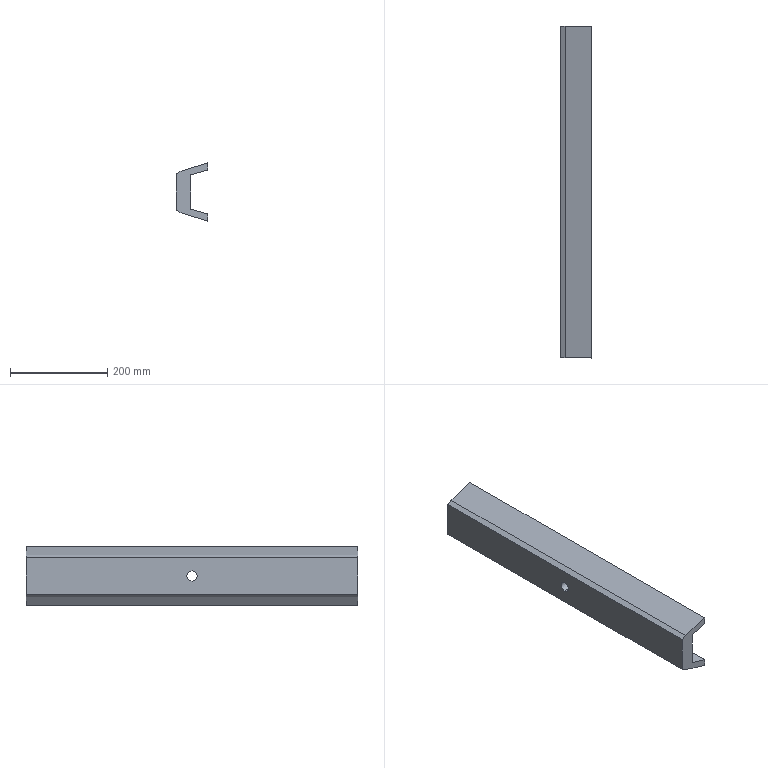Part | SolidWorks | features Extrusion 1, ICE 1 | 1 solid | 14 faces | box 65 x 682 x 120 mm | volume 2487309 mm3 | plane 12 | cylinder 2 | commonest cylinder face diameters 21 x2
STEP:
#1=CARTESIAN_POINT('',(30.,0.,-10.5));
#2=VERTEX_POINT('',#1);
#3=CARTESIAN_POINT('',(30.,0.,10.5));
#4=VERTEX_POINT('',#3);
#5=CARTESIAN_POINT('',(30.,0.,0.));
#6=DIRECTION('',(-1.,0.,0.));
#7=DIRECTION('',(0.,0.,1.));
#8=AXIS2_PLACEMENT_3D('',#5,#6,#7);
#9=CIRCLE('',#8,10.5);
#10=EDGE_CURVE('',#2,#4,#9,.T.);
#11=ORIENTED_EDGE('',*,*,#10,.F.);
#12=CARTESIAN_POINT('',(0.,0.,-10.5));
#13=VERTEX_POINT('',#12);
#14=CARTESIAN_POINT('',(95.,0.,-10.5));
#15=DIRECTION('',(-1.,0.,0.));
#16=VECTOR('',#15,1000.);
#17=LINE('',#14,#16);
#18=EDGE_CURVE('',#2,#13,#17,.T.);
#19=ORIENTED_EDGE('',*,*,#18,.T.);
#20=CARTESIAN_POINT('',(0.,0.,10.5));
#21=VERTEX_POINT('',#20);
#22=CARTESIAN_POINT('',(0.,0.,0.));
#23=DIRECTION('',(-1.,0.,0.));
#24=DIRECTION('',(0.,0.,1.));
#25=AXIS2_PLACEMENT_3D('',#22,#23,#24);
#26=CIRCLE('',#25,10.5);
#27=EDGE_CURVE('',#13,#21,#26,.T.);
#28=ORIENTED_EDGE('',*,*,#27,.T.);
#29=CARTESIAN_POINT('',(95.,0.,10.5));
#30=DIRECTION('',(-1.,0.,0.));
#31=VECTOR('',#30,1000.);
#32=LINE('',#29,#31);
#33=EDGE_CURVE('',#4,#21,#32,.T.);
#34=ORIENTED_EDGE('',*,*,#33,.F.);
#35=EDGE_LOOP('',(#11,#19,#28,#34));
#36=FACE_OUTER_BOUND('',#35,.T.);
#37=CARTESIAN_POINT('',(95.,0.,0.));
#38=DIRECTION('',(-1.,0.,0.));
#39=DIRECTION('',(0.,0.,1.));
#40=AXIS2_PLACEMENT_3D('',#37,#38,#39);
#41=CYLINDRICAL_SURFACE('',#40,10.5);
#42=ADVANCED_FACE('',(#36),#41,.F.);
#43=CARTESIAN_POINT('',(65.,-341.,45.));
#44=VERTEX_POINT('',#43);
#45=CARTESIAN_POINT('',(30.,-341.,35.));
#46=VERTEX_POINT('',#45);
#47=CARTESIAN_POINT('',(65.,-341.,45.));
#48=DIRECTION('',(-0.9615,0.,-0.2747));
#49=VECTOR('',#48,1000.);
#50=LINE('',#47,#49);
#51=EDGE_CURVE('',#44,#46,#50,.T.);
#52=ORIENTED_EDGE('',*,*,#51,.T.);
#53=CARTESIAN_POINT('',(30.,341.,35.));
#54=VERTEX_POINT('',#53);
#55=CARTESIAN_POINT('',(30.,341.,35.));
#56=DIRECTION('',(0.,-1.,0.));
#57=VECTOR('',#56,1000.);
#58=LINE('',#55,#57);
#59=EDGE_CURVE('',#54,#46,#58,.T.);
#60=ORIENTED_EDGE('',*,*,#59,.F.);
#61=CARTESIAN_POINT('',(65.,341.,45.));
#62=VERTEX_POINT('',#61);
#63=CARTESIAN_POINT('',(65.,341.,45.));
#64=DIRECTION('',(-0.9615,0.,-0.2747));
#65=VECTOR('',#64,1000.);
#66=LINE('',#63,#65);
#67=EDGE_CURVE('',#62,#54,#66,.T.);
#68=ORIENTED_EDGE('',*,*,#67,.F.);
#69=CARTESIAN_POINT('',(65.,341.,45.));
#70=DIRECTION('',(0.,-1.,0.));
#71=VECTOR('',#70,1000.);
#72=LINE('',#69,#71);
#73=EDGE_CURVE('',#62,#44,#72,.T.);
#74=ORIENTED_EDGE('',*,*,#73,.T.);
#75=EDGE_LOOP('',(#52,#60,#68,#74));
#76=FACE_OUTER_BOUND('',#75,.T.);
#77=CARTESIAN_POINT('',(65.,341.,45.));
#78=DIRECTION('',(-0.2747,0.,0.9615));
#79=DIRECTION('',(0.9615,0.,0.2747));
#80=AXIS2_PLACEMENT_3D('',#77,#78,#79);
#81=PLANE('',#80);
#82=ADVANCED_FACE('',(#76),#81,.F.);
#83=CARTESIAN_POINT('',(30.,0.,0.));
#84=DIRECTION('',(-1.,0.,0.));
#85=DIRECTION('',(0.,0.,1.));
#86=AXIS2_PLACEMENT_3D('',#83,#84,#85);
#87=CIRCLE('',#86,10.5);
#88=EDGE_CURVE('',#4,#2,#87,.T.);
#89=ORIENTED_EDGE('',*,*,#88,.T.);
#90=ORIENTED_EDGE('',*,*,#10,.T.);
#91=EDGE_LOOP('',(#89,#90));
#92=FACE_BOUND('',#91,.T.);
#93=CARTESIAN_POINT('',(30.,-341.,-35.));
#94=VERTEX_POINT('',#93);
#95=CARTESIAN_POINT('',(30.,-341.,-35.));
#96=DIRECTION('',(0.,0.,-1.));
#97=VECTOR('',#96,1000.);
#98=LINE('',#95,#97);
#99=EDGE_CURVE('',#46,#94,#98,.T.);
#100=ORIENTED_EDGE('',*,*,#99,.T.);
#101=CARTESIAN_POINT('',(30.,341.,-35.));
#102=VERTEX_POINT('',#101);
#103=CARTESIAN_POINT('',(30.,341.,-35.));
#104=DIRECTION('',(0.,-1.,0.));
#105=VECTOR('',#104,1000.);
#106=LINE('',#103,#105);
#107=EDGE_CURVE('',#102,#94,#106,.T.);
#108=ORIENTED_EDGE('',*,*,#107,.F.);
#109=CARTESIAN_POINT('',(30.,341.,-35.));
#110=DIRECTION('',(0.,0.,-1.));
#111=VECTOR('',#110,1000.);
#112=LINE('',#109,#111);
#113=EDGE_CURVE('',#54,#102,#112,.T.);
#114=ORIENTED_EDGE('',*,*,#113,.F.);
#115=ORIENTED_EDGE('',*,*,#59,.T.);
#116=EDGE_LOOP('',(#100,#108,#114,#115));
#117=FACE_OUTER_BOUND('',#116,.T.);
#118=CARTESIAN_POINT('',(30.,341.,-35.));
#119=DIRECTION('',(-1.,0.,0.));
#120=DIRECTION('',(0.,0.,1.));
#121=AXIS2_PLACEMENT_3D('',#118,#119,#120);
#122=PLANE('',#121);
#123=ADVANCED_FACE('',(#92,#117),#122,.F.);
#124=CARTESIAN_POINT('',(65.,-341.,-45.));
#125=VERTEX_POINT('',#124);
#126=CARTESIAN_POINT('',(65.,-341.,-45.));
#127=DIRECTION('',(0.9615,0.,-0.2747));
#128=VECTOR('',#127,1000.);
#129=LINE('',#126,#128);
#130=EDGE_CURVE('',#94,#125,#129,.T.);
#131=ORIENTED_EDGE('',*,*,#130,.T.);
#132=CARTESIAN_POINT('',(65.,341.,-45.));
#133=VERTEX_POINT('',#132);
#134=CARTESIAN_POINT('',(65.,341.,-45.));
#135=DIRECTION('',(0.,-1.,0.));
#136=VECTOR('',#135,1000.);
#137=LINE('',#134,#136);
#138=EDGE_CURVE('',#133,#125,#137,.T.);
#139=ORIENTED_EDGE('',*,*,#138,.F.);
#140=CARTESIAN_POINT('',(65.,341.,-45.));
#141=DIRECTION('',(0.9615,0.,-0.2747));
#142=VECTOR('',#141,1000.);
#143=LINE('',#140,#142);
#144=EDGE_CURVE('',#102,#133,#143,.T.);
#145=ORIENTED_EDGE('',*,*,#144,.F.);
#146=ORIENTED_EDGE('',*,*,#107,.T.);
#147=EDGE_LOOP('',(#131,#139,#145,#146));
#148=FACE_OUTER_BOUND('',#147,.T.);
#149=CARTESIAN_POINT('',(65.,341.,-45.));
#150=DIRECTION('',(-0.2747,0.,-0.9615));
#151=DIRECTION('',(-0.9615,0.,0.2747));
#152=AXIS2_PLACEMENT_3D('',#149,#150,#151);
#153=PLANE('',#152);
#154=ADVANCED_FACE('',(#148),#153,.F.);
#155=CARTESIAN_POINT('',(65.,-341.,-60.));
#156=VERTEX_POINT('',#155);
#157=CARTESIAN_POINT('',(65.,-341.,-60.));
#158=DIRECTION('',(0.,0.,-1.));
#159=VECTOR('',#158,1000.);
#160=LINE('',#157,#159);
#161=EDGE_CURVE('',#125,#156,#160,.T.);
#162=ORIENTED_EDGE('',*,*,#161,.T.);
#163=CARTESIAN_POINT('',(65.,341.,-60.));
#164=VERTEX_POINT('',#163);
#165=CARTESIAN_POINT('',(65.,341.,-60.));
#166=DIRECTION('',(0.,-1.,0.));
#167=VECTOR('',#166,1000.);
#168=LINE('',#165,#167);
#169=EDGE_CURVE('',#164,#156,#168,.T.);
#170=ORIENTED_EDGE('',*,*,#169,.F.);
#171=CARTESIAN_POINT('',(65.,341.,-60.));
#172=DIRECTION('',(0.,0.,-1.));
#173=VECTOR('',#172,1000.);
#174=LINE('',#171,#173);
#175=EDGE_CURVE('',#133,#164,#174,.T.);
#176=ORIENTED_EDGE('',*,*,#175,.F.);
#177=ORIENTED_EDGE('',*,*,#138,.T.);
#178=EDGE_LOOP('',(#162,#170,#176,#177));
#179=FACE_OUTER_BOUND('',#178,.T.);
#180=CARTESIAN_POINT('',(65.,341.,-60.));
#181=DIRECTION('',(-1.,0.,0.));
#182=DIRECTION('',(0.,0.,1.));
#183=AXIS2_PLACEMENT_3D('',#180,#181,#182);
#184=PLANE('',#183);
#185=ADVANCED_FACE('',(#179),#184,.F.);
#186=CARTESIAN_POINT('',(10.,-341.,-42.882));
#187=VERTEX_POINT('',#186);
#188=CARTESIAN_POINT('',(10.,-341.,-42.882));
#189=DIRECTION('',(-0.9548,0.,0.2972));
#190=VECTOR('',#189,1000.);
#191=LINE('',#188,#190);
#192=EDGE_CURVE('',#156,#187,#191,.T.);
#193=ORIENTED_EDGE('',*,*,#192,.T.);
#194=CARTESIAN_POINT('',(10.,341.,-42.882));
#195=VERTEX_POINT('',#194);
#196=CARTESIAN_POINT('',(10.,341.,-42.882));
#197=DIRECTION('',(0.,-1.,0.));
#198=VECTOR('',#197,1000.);
#199=LINE('',#196,#198);
#200=EDGE_CURVE('',#195,#187,#199,.T.);
#201=ORIENTED_EDGE('',*,*,#200,.F.);
#202=CARTESIAN_POINT('',(10.,341.,-42.882));
#203=DIRECTION('',(-0.9548,0.,0.2972));
#204=VECTOR('',#203,1000.);
#205=LINE('',#202,#204);
#206=EDGE_CURVE('',#164,#195,#205,.T.);
#207=ORIENTED_EDGE('',*,*,#206,.F.);
#208=ORIENTED_EDGE('',*,*,#169,.T.);
#209=EDGE_LOOP('',(#193,#201,#207,#208));
#210=FACE_OUTER_BOUND('',#209,.T.);
#211=CARTESIAN_POINT('',(10.,341.,-42.882));
#212=DIRECTION('',(0.2972,0.,0.9548));
#213=DIRECTION('',(0.9548,0.,-0.2972));
#214=AXIS2_PLACEMENT_3D('',#211,#212,#213);
#215=PLANE('',#214);
#216=ADVANCED_FACE('',(#210),#215,.F.);
#217=CARTESIAN_POINT('',(0.,-341.,-37.5));
#218=VERTEX_POINT('',#217);
#219=CARTESIAN_POINT('',(0.,-341.,-37.5));
#220=DIRECTION('',(-0.8806,0.,0.4739));
#221=VECTOR('',#220,1000.);
#222=LINE('',#219,#221);
#223=EDGE_CURVE('',#187,#218,#222,.T.);
#224=ORIENTED_EDGE('',*,*,#223,.T.);
#225=CARTESIAN_POINT('',(0.,341.,-37.5));
#226=VERTEX_POINT('',#225);
#227=CARTESIAN_POINT('',(0.,341.,-37.5));
#228=DIRECTION('',(0.,-1.,0.));
#229=VECTOR('',#228,1000.);
#230=LINE('',#227,#229);
#231=EDGE_CURVE('',#226,#218,#230,.T.);
#232=ORIENTED_EDGE('',*,*,#231,.F.);
#233=CARTESIAN_POINT('',(0.,341.,-37.5));
#234=DIRECTION('',(-0.8806,0.,0.4739));
#235=VECTOR('',#234,1000.);
#236=LINE('',#233,#235);
#237=EDGE_CURVE('',#195,#226,#236,.T.);
#238=ORIENTED_EDGE('',*,*,#237,.F.);
#239=ORIENTED_EDGE('',*,*,#200,.T.);
#240=EDGE_LOOP('',(#224,#232,#238,#239));
#241=FACE_OUTER_BOUND('',#240,.T.);
#242=CARTESIAN_POINT('',(0.,341.,-37.5));
#243=DIRECTION('',(0.4739,0.,0.8806));
#244=DIRECTION('',(0.8806,0.,-0.4739));
#245=AXIS2_PLACEMENT_3D('',#242,#243,#244);
#246=PLANE('',#245);
#247=ADVANCED_FACE('',(#241),#246,.F.);
#248=CARTESIAN_POINT('',(0.,0.,0.));
#249=DIRECTION('',(-1.,0.,0.));
#250=DIRECTION('',(0.,0.,1.));
#251=AXIS2_PLACEMENT_3D('',#248,#249,#250);
#252=CIRCLE('',#251,10.5);
#253=EDGE_CURVE('',#21,#13,#252,.T.);
#254=ORIENTED_EDGE('',*,*,#253,.F.);
#255=ORIENTED_EDGE('',*,*,#27,.F.);
#256=EDGE_LOOP('',(#254,#255));
#257=FACE_BOUND('',#256,.T.);
#258=CARTESIAN_POINT('',(0.,-341.,37.5));
#259=VERTEX_POINT('',#258);
#260=CARTESIAN_POINT('',(0.,-341.,37.5));
#261=DIRECTION('',(0.,0.,1.));
#262=VECTOR('',#261,1000.);
#263=LINE('',#260,#262);
#264=EDGE_CURVE('',#218,#259,#263,.T.);
#265=ORIENTED_EDGE('',*,*,#264,.T.);
#266=CARTESIAN_POINT('',(0.,341.,37.5));
#267=VERTEX_POINT('',#266);
#268=CARTESIAN_POINT('',(0.,341.,37.5));
#269=DIRECTION('',(0.,-1.,0.));
#270=VECTOR('',#269,1000.);
#271=LINE('',#268,#270);
#272=EDGE_CURVE('',#267,#259,#271,.T.);
#273=ORIENTED_EDGE('',*,*,#272,.F.);
#274=CARTESIAN_POINT('',(0.,341.,37.5));
#275=DIRECTION('',(0.,0.,1.));
#276=VECTOR('',#275,1000.);
#277=LINE('',#274,#276);
#278=EDGE_CURVE('',#226,#267,#277,.T.);
#279=ORIENTED_EDGE('',*,*,#278,.F.);
#280=ORIENTED_EDGE('',*,*,#231,.T.);
#281=EDGE_LOOP('',(#265,#273,#279,#280));
#282=FACE_OUTER_BOUND('',#281,.T.);
#283=CARTESIAN_POINT('',(0.,341.,37.5));
#284=DIRECTION('',(1.,0.,0.));
#285=DIRECTION('',(0.,0.,-1.));
#286=AXIS2_PLACEMENT_3D('',#283,#284,#285);
#287=PLANE('',#286);
#288=ADVANCED_FACE('',(#257,#282),#287,.F.);
#289=CARTESIAN_POINT('',(10.,-341.,42.882));
#290=VERTEX_POINT('',#289);
#291=CARTESIAN_POINT('',(0.,-341.,37.5));
#292=DIRECTION('',(0.8806,0.,0.4739));
#293=VECTOR('',#292,1000.);
#294=LINE('',#291,#293);
#295=EDGE_CURVE('',#259,#290,#294,.T.);
#296=ORIENTED_EDGE('',*,*,#295,.T.);
#297=CARTESIAN_POINT('',(10.,341.,42.882));
#298=VERTEX_POINT('',#297);
#299=CARTESIAN_POINT('',(10.,341.,42.882));
#300=DIRECTION('',(0.,-1.,0.));
#301=VECTOR('',#300,1000.);
#302=LINE('',#299,#301);
#303=EDGE_CURVE('',#298,#290,#302,.T.);
#304=ORIENTED_EDGE('',*,*,#303,.F.);
#305=CARTESIAN_POINT('',(0.,341.,37.5));
#306=DIRECTION('',(0.8806,0.,0.4739));
#307=VECTOR('',#306,1000.);
#308=LINE('',#305,#307);
#309=EDGE_CURVE('',#267,#298,#308,.T.);
#310=ORIENTED_EDGE('',*,*,#309,.F.);
#311=ORIENTED_EDGE('',*,*,#272,.T.);
#312=EDGE_LOOP('',(#296,#304,#310,#311));
#313=FACE_OUTER_BOUND('',#312,.T.);
#314=CARTESIAN_POINT('',(0.,341.,37.5));
#315=DIRECTION('',(0.4739,0.,-0.8806));
#316=DIRECTION('',(-0.8806,0.,-0.4739));
#317=AXIS2_PLACEMENT_3D('',#314,#315,#316);
#318=PLANE('',#317);
#319=ADVANCED_FACE('',(#313),#318,.F.);
#320=CARTESIAN_POINT('',(65.,-341.,60.));
#321=VERTEX_POINT('',#320);
#322=CARTESIAN_POINT('',(10.,-341.,42.882));
#323=DIRECTION('',(0.9548,0.,0.2972));
#324=VECTOR('',#323,1000.);
#325=LINE('',#322,#324);
#326=EDGE_CURVE('',#290,#321,#325,.T.);
#327=ORIENTED_EDGE('',*,*,#326,.T.);
#328=CARTESIAN_POINT('',(65.,341.,60.));
#329=VERTEX_POINT('',#328);
#330=CARTESIAN_POINT('',(65.,341.,60.));
#331=DIRECTION('',(0.,-1.,0.));
#332=VECTOR('',#331,1000.);
#333=LINE('',#330,#332);
#334=EDGE_CURVE('',#329,#321,#333,.T.);
#335=ORIENTED_EDGE('',*,*,#334,.F.);
#336=CARTESIAN_POINT('',(10.,341.,42.882));
#337=DIRECTION('',(0.9548,0.,0.2972));
#338=VECTOR('',#337,1000.);
#339=LINE('',#336,#338);
#340=EDGE_CURVE('',#298,#329,#339,.T.);
#341=ORIENTED_EDGE('',*,*,#340,.F.);
#342=ORIENTED_EDGE('',*,*,#303,.T.);
#343=EDGE_LOOP('',(#327,#335,#341,#342));
#344=FACE_OUTER_BOUND('',#343,.T.);
#345=CARTESIAN_POINT('',(10.,341.,42.882));
#346=DIRECTION('',(0.2972,0.,-0.9548));
#347=DIRECTION('',(-0.9548,0.,-0.2972));
#348=AXIS2_PLACEMENT_3D('',#345,#346,#347);
#349=PLANE('',#348);
#350=ADVANCED_FACE('',(#344),#349,.F.);
#351=CARTESIAN_POINT('',(65.,-341.,60.));
#352=DIRECTION('',(0.,0.,-1.));
#353=VECTOR('',#352,1000.);
#354=LINE('',#351,#353);
#355=EDGE_CURVE('',#321,#44,#354,.T.);
#356=ORIENTED_EDGE('',*,*,#355,.T.);
#357=ORIENTED_EDGE('',*,*,#73,.F.);
#358=CARTESIAN_POINT('',(65.,341.,60.));
#359=DIRECTION('',(0.,0.,-1.));
#360=VECTOR('',#359,1000.);
#361=LINE('',#358,#360);
#362=EDGE_CURVE('',#329,#62,#361,.T.);
#363=ORIENTED_EDGE('',*,*,#362,.F.);
#364=ORIENTED_EDGE('',*,*,#334,.T.);
#365=EDGE_LOOP('',(#356,#357,#363,#364));
#366=FACE_OUTER_BOUND('',#365,.T.);
#367=CARTESIAN_POINT('',(65.,341.,60.));
#368=DIRECTION('',(-1.,0.,0.));
#369=DIRECTION('',(0.,0.,1.));
#370=AXIS2_PLACEMENT_3D('',#367,#368,#369);
#371=PLANE('',#370);
#372=ADVANCED_FACE('',(#366),#371,.F.);
#373=ORIENTED_EDGE('',*,*,#67,.T.);
#374=ORIENTED_EDGE('',*,*,#113,.T.);
#375=ORIENTED_EDGE('',*,*,#144,.T.);
#376=ORIENTED_EDGE('',*,*,#175,.T.);
#377=ORIENTED_EDGE('',*,*,#206,.T.);
#378=ORIENTED_EDGE('',*,*,#237,.T.);
#379=ORIENTED_EDGE('',*,*,#278,.T.);
#380=ORIENTED_EDGE('',*,*,#309,.T.);
#381=ORIENTED_EDGE('',*,*,#340,.T.);
#382=ORIENTED_EDGE('',*,*,#362,.T.);
#383=EDGE_LOOP('',(#373,#374,#375,#376,#377,#378,#379,#380,#381,#382));
#384=FACE_OUTER_BOUND('',#383,.T.);
#385=CARTESIAN_POINT('',(0.,341.,0.));
#386=DIRECTION('',(0.,1.,0.));
#387=DIRECTION('',(0.,0.,1.));
#388=AXIS2_PLACEMENT_3D('',#385,#386,#387);
#389=PLANE('',#388);
#390=ADVANCED_FACE('',(#384),#389,.T.);
#391=ORIENTED_EDGE('',*,*,#51,.F.);
#392=ORIENTED_EDGE('',*,*,#355,.F.);
#393=ORIENTED_EDGE('',*,*,#326,.F.);
#394=ORIENTED_EDGE('',*,*,#295,.F.);
#395=ORIENTED_EDGE('',*,*,#264,.F.);
#396=ORIENTED_EDGE('',*,*,#223,.F.);
#397=ORIENTED_EDGE('',*,*,#192,.F.);
#398=ORIENTED_EDGE('',*,*,#161,.F.);
#399=ORIENTED_EDGE('',*,*,#130,.F.);
#400=ORIENTED_EDGE('',*,*,#99,.F.);
#401=EDGE_LOOP('',(#391,#392,#393,#394,#395,#396,#397,#398,#399,#400));
#402=FACE_OUTER_BOUND('',#401,.T.);
#403=CARTESIAN_POINT('',(0.,-341.,0.));
#404=DIRECTION('',(0.,1.,0.));
#405=DIRECTION('',(0.,0.,1.));
#406=AXIS2_PLACEMENT_3D('',#403,#404,#405);
#407=PLANE('',#406);
#408=ADVANCED_FACE('',(#402),#407,.F.);
#409=ORIENTED_EDGE('',*,*,#18,.F.);
#410=ORIENTED_EDGE('',*,*,#88,.F.);
#411=ORIENTED_EDGE('',*,*,#33,.T.);
#412=ORIENTED_EDGE('',*,*,#253,.T.);
#413=EDGE_LOOP('',(#409,#410,#411,#412));
#414=FACE_OUTER_BOUND('',#413,.T.);
#415=CARTESIAN_POINT('',(95.,0.,0.));
#416=DIRECTION('',(-1.,0.,0.));
#417=DIRECTION('',(0.,0.,1.));
#418=AXIS2_PLACEMENT_3D('',#415,#416,#417);
#419=CYLINDRICAL_SURFACE('',#418,10.5);
#420=ADVANCED_FACE('',(#414),#419,.F.);
#421=CLOSED_SHELL('',(#42,#82,#123,#154,#185,#216,#247,#288,#319,#350,#372,#390,#408,#420));
#422=MANIFOLD_SOLID_BREP('',#421);
#423=CARTESIAN_POINT('',(0.,0.,0.));
#424=DIRECTION('',(0.,0.,1.));
#425=DIRECTION('',(1.,0.,0.));
#426=AXIS2_PLACEMENT_3D('',#423,#424,#425);
#427=(LENGTH_UNIT()NAMED_UNIT(*)SI_UNIT(.MILLI.,.METRE.));
#428=UNCERTAINTY_MEASURE_WITH_UNIT(LENGTH_MEASURE(0.00001),#427,'','');
#429=(NAMED_UNIT(*)PLANE_ANGLE_UNIT()SI_UNIT($,.RADIAN.));
#430=(NAMED_UNIT(*)SI_UNIT($,.STERADIAN.)SOLID_ANGLE_UNIT());
#431=(GEOMETRIC_REPRESENTATION_CONTEXT(3)GLOBAL_UNCERTAINTY_ASSIGNED_CONTEXT((#428))GLOBAL_UNIT_ASSIGNED_CONTEXT((#427,#429,#430))REPRESENTATION_CONTEXT('',''));
#432=ADVANCED_BREP_SHAPE_REPRESENTATION('',(#422,#426),#431);